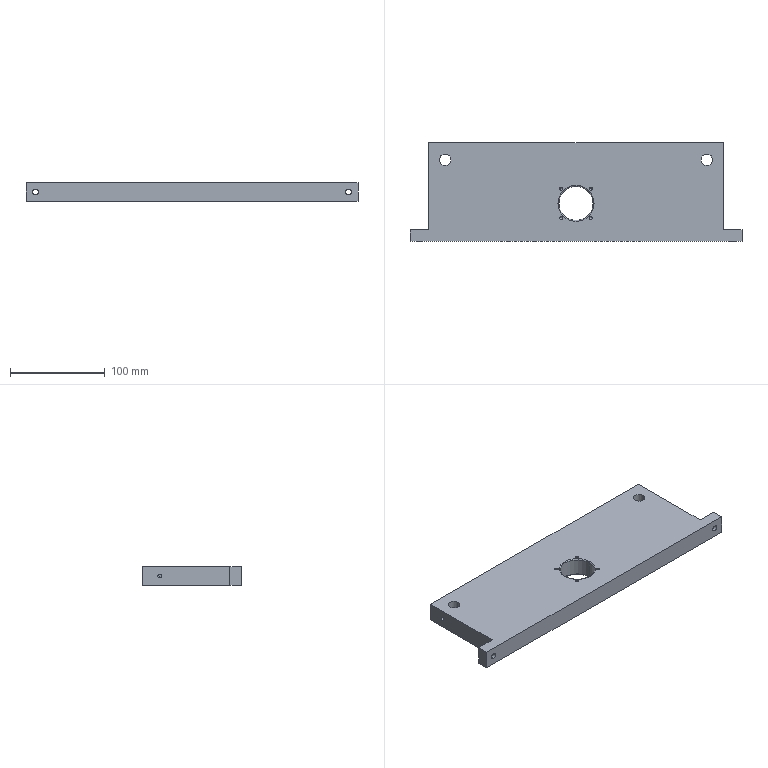Part | STEP file | 0230_204_Block | 1 solid | 48 faces | box 350 x 104 x 20 mm | volume 627795 mm3 | cylinder 26 | plane 10 | cone 8 | torus 4 | commonest cylinder face diameters 3.3 x8 4.2 x8 6 x4 12 x4 36 x2